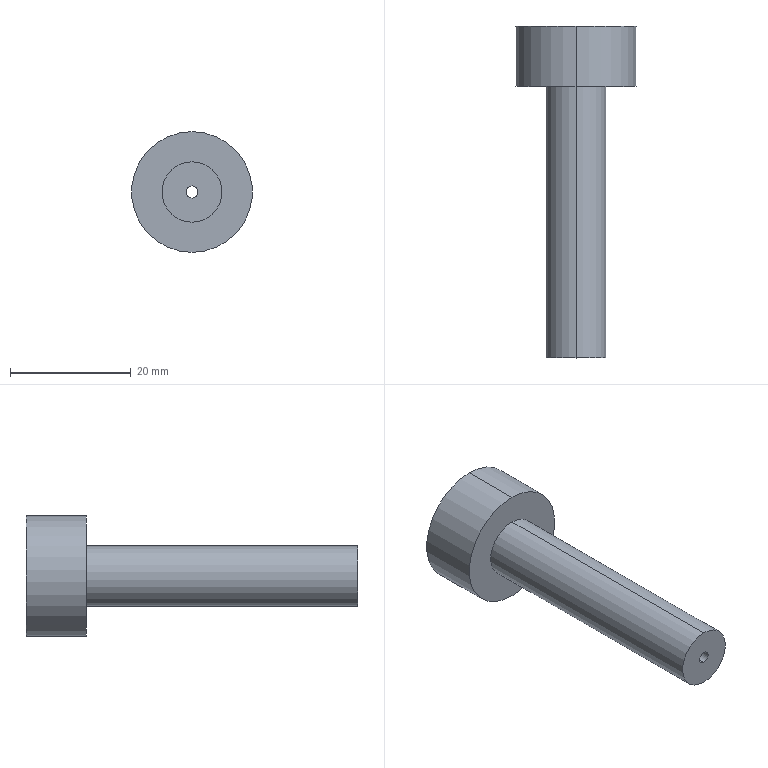Part | 1 solid | 16 faces | box 20 x 55 x 20 mm | volume 5586 mm3 | cylinder 10 | plane 4 | cone 2 | commonest cylinder face diameters 2 x4 6 x2 10 x2 20 x2
STEP:
#1=CARTESIAN_POINT('',(0.,-2.8,-1.));
#2=VERTEX_POINT('',#1);
#3=CARTESIAN_POINT('',(-1.,-2.8,0.));
#4=VERTEX_POINT('',#3);
#5=CARTESIAN_POINT('',(0.,-2.8,0.));
#6=DIRECTION('',(0.,1.,0.));
#7=DIRECTION('',(-1.,0.,0.));
#8=AXIS2_PLACEMENT_3D('',#5,#6,#7);
#9=CIRCLE('',#8,1.);
#10=EDGE_CURVE('',#2,#4,#9,.T.);
#11=ORIENTED_EDGE('',*,*,#10,.T.);
#12=CARTESIAN_POINT('',(-3.,-4.,0.));
#13=VERTEX_POINT('',#12);
#14=CARTESIAN_POINT('',(-1.,-2.8,0.));
#15=DIRECTION('',(-0.8575,-0.5145,0.));
#16=VECTOR('',#15,1000.);
#17=LINE('',#14,#16);
#18=EDGE_CURVE('',#4,#13,#17,.T.);
#19=ORIENTED_EDGE('',*,*,#18,.T.);
#20=CARTESIAN_POINT('',(0.,-4.,-3.));
#21=VERTEX_POINT('',#20);
#22=CARTESIAN_POINT('',(0.,-4.,0.));
#23=DIRECTION('',(0.,1.,0.));
#24=DIRECTION('',(-1.,0.,0.));
#25=AXIS2_PLACEMENT_3D('',#22,#23,#24);
#26=CIRCLE('',#25,3.);
#27=EDGE_CURVE('',#21,#13,#26,.T.);
#28=ORIENTED_EDGE('',*,*,#27,.F.);
#29=CARTESIAN_POINT('',(3.,-4.,0.));
#30=VERTEX_POINT('',#29);
#31=CARTESIAN_POINT('',(0.,-4.,0.));
#32=DIRECTION('',(0.,1.,0.));
#33=DIRECTION('',(-1.,0.,0.));
#34=AXIS2_PLACEMENT_3D('',#31,#32,#33);
#35=CIRCLE('',#34,3.);
#36=EDGE_CURVE('',#30,#21,#35,.T.);
#37=ORIENTED_EDGE('',*,*,#36,.F.);
#38=CARTESIAN_POINT('',(1.,-2.8,0.));
#39=VERTEX_POINT('',#38);
#40=CARTESIAN_POINT('',(1.,-2.8,0.));
#41=DIRECTION('',(0.8575,-0.5145,0.));
#42=VECTOR('',#41,1000.);
#43=LINE('',#40,#42);
#44=EDGE_CURVE('',#39,#30,#43,.T.);
#45=ORIENTED_EDGE('',*,*,#44,.F.);
#46=CARTESIAN_POINT('',(0.,-2.8,0.));
#47=DIRECTION('',(0.,1.,0.));
#48=DIRECTION('',(-1.,0.,0.));
#49=AXIS2_PLACEMENT_3D('',#46,#47,#48);
#50=CIRCLE('',#49,1.);
#51=EDGE_CURVE('',#39,#2,#50,.T.);
#52=ORIENTED_EDGE('',*,*,#51,.T.);
#53=EDGE_LOOP('',(#11,#19,#28,#37,#45,#52));
#54=FACE_OUTER_BOUND('',#53,.T.);
#55=CARTESIAN_POINT('',(0.,-2.8,0.));
#56=DIRECTION('',(0.,-1.,0.));
#57=DIRECTION('',(1.,0.,0.));
#58=AXIS2_PLACEMENT_3D('',#55,#56,#57);
#59=CONICAL_SURFACE('',#58,1.,1.03);
#60=ADVANCED_FACE('',(#54),#59,.F.);
#61=ORIENTED_EDGE('',*,*,#27,.T.);
#62=CARTESIAN_POINT('',(0.,-4.,3.));
#63=VERTEX_POINT('',#62);
#64=CARTESIAN_POINT('',(0.,-4.,0.));
#65=DIRECTION('',(0.,1.,0.));
#66=DIRECTION('',(-1.,0.,0.));
#67=AXIS2_PLACEMENT_3D('',#64,#65,#66);
#68=CIRCLE('',#67,3.);
#69=EDGE_CURVE('',#13,#63,#68,.T.);
#70=ORIENTED_EDGE('',*,*,#69,.T.);
#71=CARTESIAN_POINT('',(0.,-40.,3.));
#72=VERTEX_POINT('',#71);
#73=CARTESIAN_POINT('',(0.,-4.,3.));
#74=DIRECTION('',(0.,-1.,0.));
#75=VECTOR('',#74,1000.);
#76=LINE('',#73,#75);
#77=EDGE_CURVE('',#63,#72,#76,.T.);
#78=ORIENTED_EDGE('',*,*,#77,.T.);
#79=CARTESIAN_POINT('',(0.,-40.,-3.));
#80=VERTEX_POINT('',#79);
#81=CARTESIAN_POINT('',(0.,-40.,0.));
#82=DIRECTION('',(0.,-1.,0.));
#83=DIRECTION('',(0.,0.,-1.));
#84=AXIS2_PLACEMENT_3D('',#81,#82,#83);
#85=CIRCLE('',#84,3.);
#86=EDGE_CURVE('',#72,#80,#85,.T.);
#87=ORIENTED_EDGE('',*,*,#86,.T.);
#88=CARTESIAN_POINT('',(0.,-4.,-3.));
#89=DIRECTION('',(0.,-1.,0.));
#90=VECTOR('',#89,1000.);
#91=LINE('',#88,#90);
#92=EDGE_CURVE('',#21,#80,#91,.T.);
#93=ORIENTED_EDGE('',*,*,#92,.F.);
#94=EDGE_LOOP('',(#61,#70,#78,#87,#93));
#95=FACE_OUTER_BOUND('',#94,.T.);
#96=CARTESIAN_POINT('',(0.,-4.,0.));
#97=DIRECTION('',(0.,-1.,0.));
#98=DIRECTION('',(0.,0.,-1.));
#99=AXIS2_PLACEMENT_3D('',#96,#97,#98);
#100=CYLINDRICAL_SURFACE('',#99,3.);
#101=ADVANCED_FACE('',(#95),#100,.F.);
#102=CARTESIAN_POINT('',(0.,-45.,-1.));
#103=VERTEX_POINT('',#102);
#104=CARTESIAN_POINT('',(0.,-45.,1.));
#105=VERTEX_POINT('',#104);
#106=CARTESIAN_POINT('',(0.,-45.,0.));
#107=DIRECTION('',(0.,1.,0.));
#108=DIRECTION('',(0.,0.,1.));
#109=AXIS2_PLACEMENT_3D('',#106,#107,#108);
#110=CIRCLE('',#109,1.);
#111=EDGE_CURVE('',#103,#105,#110,.T.);
#112=ORIENTED_EDGE('',*,*,#111,.F.);
#113=CARTESIAN_POINT('',(0.,-40.,-1.));
#114=VERTEX_POINT('',#113);
#115=CARTESIAN_POINT('',(0.,-45.,-1.));
#116=DIRECTION('',(0.,1.,0.));
#117=VECTOR('',#116,1000.);
#118=LINE('',#115,#117);
#119=EDGE_CURVE('',#103,#114,#118,.T.);
#120=ORIENTED_EDGE('',*,*,#119,.T.);
#121=CARTESIAN_POINT('',(0.,-40.,1.));
#122=VERTEX_POINT('',#121);
#123=CARTESIAN_POINT('',(0.,-40.,0.));
#124=DIRECTION('',(0.,1.,0.));
#125=DIRECTION('',(0.,0.,-1.));
#126=AXIS2_PLACEMENT_3D('',#123,#124,#125);
#127=CIRCLE('',#126,1.);
#128=EDGE_CURVE('',#114,#122,#127,.T.);
#129=ORIENTED_EDGE('',*,*,#128,.T.);
#130=CARTESIAN_POINT('',(0.,-45.,1.));
#131=DIRECTION('',(0.,1.,0.));
#132=VECTOR('',#131,1000.);
#133=LINE('',#130,#132);
#134=EDGE_CURVE('',#105,#122,#133,.T.);
#135=ORIENTED_EDGE('',*,*,#134,.F.);
#136=EDGE_LOOP('',(#112,#120,#129,#135));
#137=FACE_OUTER_BOUND('',#136,.T.);
#138=CARTESIAN_POINT('',(0.,-45.,0.));
#139=DIRECTION('',(0.,1.,0.));
#140=DIRECTION('',(0.,0.,1.));
#141=AXIS2_PLACEMENT_3D('',#138,#139,#140);
#142=CYLINDRICAL_SURFACE('',#141,1.);
#143=ADVANCED_FACE('',(#137),#142,.F.);
#144=CARTESIAN_POINT('',(0.,-45.,-5.));
#145=VERTEX_POINT('',#144);
#146=CARTESIAN_POINT('',(0.,-45.,5.));
#147=VERTEX_POINT('',#146);
#148=CARTESIAN_POINT('',(0.,-45.,0.));
#149=DIRECTION('',(0.,-1.,0.));
#150=DIRECTION('',(0.,0.,-1.));
#151=AXIS2_PLACEMENT_3D('',#148,#149,#150);
#152=CIRCLE('',#151,5.);
#153=EDGE_CURVE('',#145,#147,#152,.T.);
#154=ORIENTED_EDGE('',*,*,#153,.F.);
#155=CARTESIAN_POINT('',(0.,0.,-5.));
#156=VERTEX_POINT('',#155);
#157=CARTESIAN_POINT('',(0.,-45.,-5.));
#158=DIRECTION('',(0.,1.,0.));
#159=VECTOR('',#158,1000.);
#160=LINE('',#157,#159);
#161=EDGE_CURVE('',#145,#156,#160,.T.);
#162=ORIENTED_EDGE('',*,*,#161,.T.);
#163=CARTESIAN_POINT('',(0.,0.,5.));
#164=VERTEX_POINT('',#163);
#165=CARTESIAN_POINT('',(0.,0.,0.));
#166=DIRECTION('',(0.,-1.,0.));
#167=DIRECTION('',(0.,0.,-1.));
#168=AXIS2_PLACEMENT_3D('',#165,#166,#167);
#169=CIRCLE('',#168,5.);
#170=EDGE_CURVE('',#156,#164,#169,.T.);
#171=ORIENTED_EDGE('',*,*,#170,.T.);
#172=CARTESIAN_POINT('',(0.,-45.,5.));
#173=DIRECTION('',(0.,1.,0.));
#174=VECTOR('',#173,1000.);
#175=LINE('',#172,#174);
#176=EDGE_CURVE('',#147,#164,#175,.T.);
#177=ORIENTED_EDGE('',*,*,#176,.F.);
#178=EDGE_LOOP('',(#154,#162,#171,#177));
#179=FACE_OUTER_BOUND('',#178,.T.);
#180=CARTESIAN_POINT('',(0.,-45.,0.));
#181=DIRECTION('',(0.,1.,0.));
#182=DIRECTION('',(0.,0.,1.));
#183=AXIS2_PLACEMENT_3D('',#180,#181,#182);
#184=CYLINDRICAL_SURFACE('',#183,5.);
#185=ADVANCED_FACE('',(#179),#184,.T.);
#186=CARTESIAN_POINT('',(0.,10.,10.));
#187=VERTEX_POINT('',#186);
#188=CARTESIAN_POINT('',(0.,10.,-10.));
#189=VERTEX_POINT('',#188);
#190=CARTESIAN_POINT('',(0.,10.,0.));
#191=DIRECTION('',(0.,1.,0.));
#192=DIRECTION('',(0.,0.,1.));
#193=AXIS2_PLACEMENT_3D('',#190,#191,#192);
#194=CIRCLE('',#193,10.);
#195=EDGE_CURVE('',#187,#189,#194,.T.);
#196=ORIENTED_EDGE('',*,*,#195,.F.);
#197=CARTESIAN_POINT('',(0.,0.,10.));
#198=VERTEX_POINT('',#197);
#199=CARTESIAN_POINT('',(0.,10.,10.));
#200=DIRECTION('',(0.,-1.,0.));
#201=VECTOR('',#200,1000.);
#202=LINE('',#199,#201);
#203=EDGE_CURVE('',#187,#198,#202,.T.);
#204=ORIENTED_EDGE('',*,*,#203,.T.);
#205=CARTESIAN_POINT('',(0.,0.,-10.));
#206=VERTEX_POINT('',#205);
#207=CARTESIAN_POINT('',(0.,0.,0.));
#208=DIRECTION('',(0.,1.,0.));
#209=DIRECTION('',(0.,0.,1.));
#210=AXIS2_PLACEMENT_3D('',#207,#208,#209);
#211=CIRCLE('',#210,10.);
#212=EDGE_CURVE('',#198,#206,#211,.T.);
#213=ORIENTED_EDGE('',*,*,#212,.T.);
#214=CARTESIAN_POINT('',(0.,10.,-10.));
#215=DIRECTION('',(0.,-1.,0.));
#216=VECTOR('',#215,1000.);
#217=LINE('',#214,#216);
#218=EDGE_CURVE('',#189,#206,#217,.T.);
#219=ORIENTED_EDGE('',*,*,#218,.F.);
#220=EDGE_LOOP('',(#196,#204,#213,#219));
#221=FACE_OUTER_BOUND('',#220,.T.);
#222=CARTESIAN_POINT('',(0.,10.,0.));
#223=DIRECTION('',(0.,-1.,0.));
#224=DIRECTION('',(0.,0.,-1.));
#225=AXIS2_PLACEMENT_3D('',#222,#223,#224);
#226=CYLINDRICAL_SURFACE('',#225,10.);
#227=ADVANCED_FACE('',(#221),#226,.T.);
#228=ORIENTED_EDGE('',*,*,#10,.F.);
#229=CARTESIAN_POINT('',(0.,10.,-1.));
#230=VERTEX_POINT('',#229);
#231=CARTESIAN_POINT('',(0.,-45.,-1.));
#232=DIRECTION('',(0.,1.,0.));
#233=VECTOR('',#232,1000.);
#234=LINE('',#231,#233);
#235=EDGE_CURVE('',#2,#230,#234,.T.);
#236=ORIENTED_EDGE('',*,*,#235,.T.);
#237=CARTESIAN_POINT('',(0.,10.,1.));
#238=VERTEX_POINT('',#237);
#239=CARTESIAN_POINT('',(0.,10.,0.));
#240=DIRECTION('',(0.,1.,0.));
#241=DIRECTION('',(0.,0.,1.));
#242=AXIS2_PLACEMENT_3D('',#239,#240,#241);
#243=CIRCLE('',#242,1.);
#244=EDGE_CURVE('',#230,#238,#243,.T.);
#245=ORIENTED_EDGE('',*,*,#244,.T.);
#246=CARTESIAN_POINT('',(0.,-2.8,1.));
#247=VERTEX_POINT('',#246);
#248=CARTESIAN_POINT('',(0.,-45.,1.));
#249=DIRECTION('',(0.,1.,0.));
#250=VECTOR('',#249,1000.);
#251=LINE('',#248,#250);
#252=EDGE_CURVE('',#247,#238,#251,.T.);
#253=ORIENTED_EDGE('',*,*,#252,.F.);
#254=CARTESIAN_POINT('',(0.,-2.8,0.));
#255=DIRECTION('',(0.,1.,0.));
#256=DIRECTION('',(-1.,0.,0.));
#257=AXIS2_PLACEMENT_3D('',#254,#255,#256);
#258=CIRCLE('',#257,1.);
#259=EDGE_CURVE('',#4,#247,#258,.T.);
#260=ORIENTED_EDGE('',*,*,#259,.F.);
#261=EDGE_LOOP('',(#228,#236,#245,#253,#260));
#262=FACE_OUTER_BOUND('',#261,.T.);
#263=CARTESIAN_POINT('',(0.,-45.,0.));
#264=DIRECTION('',(0.,1.,0.));
#265=DIRECTION('',(0.,0.,1.));
#266=AXIS2_PLACEMENT_3D('',#263,#264,#265);
#267=CYLINDRICAL_SURFACE('',#266,1.);
#268=ADVANCED_FACE('',(#262),#267,.F.);
#269=ORIENTED_EDGE('',*,*,#235,.F.);
#270=ORIENTED_EDGE('',*,*,#51,.F.);
#271=CARTESIAN_POINT('',(0.,-2.8,0.));
#272=DIRECTION('',(0.,1.,0.));
#273=DIRECTION('',(-1.,0.,0.));
#274=AXIS2_PLACEMENT_3D('',#271,#272,#273);
#275=CIRCLE('',#274,1.);
#276=EDGE_CURVE('',#247,#39,#275,.T.);
#277=ORIENTED_EDGE('',*,*,#276,.F.);
#278=ORIENTED_EDGE('',*,*,#252,.T.);
#279=CARTESIAN_POINT('',(0.,10.,0.));
#280=DIRECTION('',(0.,1.,0.));
#281=DIRECTION('',(0.,0.,1.));
#282=AXIS2_PLACEMENT_3D('',#279,#280,#281);
#283=CIRCLE('',#282,1.);
#284=EDGE_CURVE('',#238,#230,#283,.T.);
#285=ORIENTED_EDGE('',*,*,#284,.T.);
#286=EDGE_LOOP('',(#269,#270,#277,#278,#285));
#287=FACE_OUTER_BOUND('',#286,.T.);
#288=CARTESIAN_POINT('',(0.,-45.,0.));
#289=DIRECTION('',(0.,1.,0.));
#290=DIRECTION('',(0.,0.,1.));
#291=AXIS2_PLACEMENT_3D('',#288,#289,#290);
#292=CYLINDRICAL_SURFACE('',#291,1.);
#293=ADVANCED_FACE('',(#287),#292,.F.);
#294=ORIENTED_EDGE('',*,*,#203,.F.);
#295=CARTESIAN_POINT('',(0.,10.,0.));
#296=DIRECTION('',(0.,1.,0.));
#297=DIRECTION('',(0.,0.,1.));
#298=AXIS2_PLACEMENT_3D('',#295,#296,#297);
#299=CIRCLE('',#298,10.);
#300=EDGE_CURVE('',#189,#187,#299,.T.);
#301=ORIENTED_EDGE('',*,*,#300,.F.);
#302=ORIENTED_EDGE('',*,*,#218,.T.);
#303=CARTESIAN_POINT('',(0.,0.,0.));
#304=DIRECTION('',(0.,1.,0.));
#305=DIRECTION('',(0.,0.,1.));
#306=AXIS2_PLACEMENT_3D('',#303,#304,#305);
#307=CIRCLE('',#306,10.);
#308=EDGE_CURVE('',#206,#198,#307,.T.);
#309=ORIENTED_EDGE('',*,*,#308,.T.);
#310=EDGE_LOOP('',(#294,#301,#302,#309));
#311=FACE_OUTER_BOUND('',#310,.T.);
#312=CARTESIAN_POINT('',(0.,10.,0.));
#313=DIRECTION('',(0.,-1.,0.));
#314=DIRECTION('',(0.,0.,-1.));
#315=AXIS2_PLACEMENT_3D('',#312,#313,#314);
#316=CYLINDRICAL_SURFACE('',#315,10.);
#317=ADVANCED_FACE('',(#311),#316,.T.);
#318=ORIENTED_EDGE('',*,*,#284,.F.);
#319=ORIENTED_EDGE('',*,*,#244,.F.);
#320=EDGE_LOOP('',(#318,#319));
#321=FACE_BOUND('',#320,.T.);
#322=ORIENTED_EDGE('',*,*,#300,.T.);
#323=ORIENTED_EDGE('',*,*,#195,.T.);
#324=EDGE_LOOP('',(#322,#323));
#325=FACE_OUTER_BOUND('',#324,.T.);
#326=CARTESIAN_POINT('',(0.,10.,0.));
#327=DIRECTION('',(0.,1.,0.));
#328=DIRECTION('',(0.,0.,1.));
#329=AXIS2_PLACEMENT_3D('',#326,#327,#328);
#330=PLANE('',#329);
#331=ADVANCED_FACE('',(#321,#325),#330,.T.);
#332=CARTESIAN_POINT('',(0.,0.,0.));
#333=DIRECTION('',(0.,-1.,0.));
#334=DIRECTION('',(0.,0.,-1.));
#335=AXIS2_PLACEMENT_3D('',#332,#333,#334);
#336=CIRCLE('',#335,5.);
#337=EDGE_CURVE('',#164,#156,#336,.T.);
#338=ORIENTED_EDGE('',*,*,#337,.F.);
#339=ORIENTED_EDGE('',*,*,#170,.F.);
#340=EDGE_LOOP('',(#338,#339));
#341=FACE_BOUND('',#340,.T.);
#342=ORIENTED_EDGE('',*,*,#308,.F.);
#343=ORIENTED_EDGE('',*,*,#212,.F.);
#344=EDGE_LOOP('',(#342,#343));
#345=FACE_OUTER_BOUND('',#344,.T.);
#346=CARTESIAN_POINT('',(0.,0.,0.));
#347=DIRECTION('',(0.,1.,0.));
#348=DIRECTION('',(0.,0.,1.));
#349=AXIS2_PLACEMENT_3D('',#346,#347,#348);
#350=PLANE('',#349);
#351=ADVANCED_FACE('',(#341,#345),#350,.F.);
#352=ORIENTED_EDGE('',*,*,#161,.F.);
#353=CARTESIAN_POINT('',(0.,-45.,0.));
#354=DIRECTION('',(0.,-1.,0.));
#355=DIRECTION('',(0.,0.,-1.));
#356=AXIS2_PLACEMENT_3D('',#353,#354,#355);
#357=CIRCLE('',#356,5.);
#358=EDGE_CURVE('',#147,#145,#357,.T.);
#359=ORIENTED_EDGE('',*,*,#358,.F.);
#360=ORIENTED_EDGE('',*,*,#176,.T.);
#361=ORIENTED_EDGE('',*,*,#337,.T.);
#362=EDGE_LOOP('',(#352,#359,#360,#361));
#363=FACE_OUTER_BOUND('',#362,.T.);
#364=CARTESIAN_POINT('',(0.,-45.,0.));
#365=DIRECTION('',(0.,1.,0.));
#366=DIRECTION('',(0.,0.,1.));
#367=AXIS2_PLACEMENT_3D('',#364,#365,#366);
#368=CYLINDRICAL_SURFACE('',#367,5.);
#369=ADVANCED_FACE('',(#363),#368,.T.);
#370=CARTESIAN_POINT('',(0.,-45.,0.));
#371=DIRECTION('',(0.,1.,0.));
#372=DIRECTION('',(0.,0.,1.));
#373=AXIS2_PLACEMENT_3D('',#370,#371,#372);
#374=CIRCLE('',#373,1.);
#375=EDGE_CURVE('',#105,#103,#374,.T.);
#376=ORIENTED_EDGE('',*,*,#375,.T.);
#377=ORIENTED_EDGE('',*,*,#111,.T.);
#378=EDGE_LOOP('',(#376,#377));
#379=FACE_BOUND('',#378,.T.);
#380=ORIENTED_EDGE('',*,*,#358,.T.);
#381=ORIENTED_EDGE('',*,*,#153,.T.);
#382=EDGE_LOOP('',(#380,#381));
#383=FACE_OUTER_BOUND('',#382,.T.);
#384=CARTESIAN_POINT('',(0.,-45.,0.));
#385=DIRECTION('',(0.,-1.,0.));
#386=DIRECTION('',(0.,0.,-1.));
#387=AXIS2_PLACEMENT_3D('',#384,#385,#386);
#388=PLANE('',#387);
#389=ADVANCED_FACE('',(#379,#383),#388,.T.);
#390=ORIENTED_EDGE('',*,*,#119,.F.);
#391=ORIENTED_EDGE('',*,*,#375,.F.);
#392=ORIENTED_EDGE('',*,*,#134,.T.);
#393=CARTESIAN_POINT('',(0.,-40.,0.));
#394=DIRECTION('',(0.,1.,0.));
#395=DIRECTION('',(0.,0.,-1.));
#396=AXIS2_PLACEMENT_3D('',#393,#394,#395);
#397=CIRCLE('',#396,1.);
#398=EDGE_CURVE('',#122,#114,#397,.T.);
#399=ORIENTED_EDGE('',*,*,#398,.T.);
#400=EDGE_LOOP('',(#390,#391,#392,#399));
#401=FACE_OUTER_BOUND('',#400,.T.);
#402=CARTESIAN_POINT('',(0.,-45.,0.));
#403=DIRECTION('',(0.,1.,0.));
#404=DIRECTION('',(0.,0.,1.));
#405=AXIS2_PLACEMENT_3D('',#402,#403,#404);
#406=CYLINDRICAL_SURFACE('',#405,1.);
#407=ADVANCED_FACE('',(#401),#406,.F.);
#408=CARTESIAN_POINT('',(0.,-40.,0.));
#409=DIRECTION('',(0.,-1.,0.));
#410=DIRECTION('',(0.,0.,-1.));
#411=AXIS2_PLACEMENT_3D('',#408,#409,#410);
#412=CIRCLE('',#411,3.);
#413=EDGE_CURVE('',#80,#72,#412,.T.);
#414=ORIENTED_EDGE('',*,*,#413,.F.);
#415=ORIENTED_EDGE('',*,*,#86,.F.);
#416=EDGE_LOOP('',(#414,#415));
#417=FACE_OUTER_BOUND('',#416,.T.);
#418=ORIENTED_EDGE('',*,*,#398,.F.);
#419=ORIENTED_EDGE('',*,*,#128,.F.);
#420=EDGE_LOOP('',(#418,#419));
#421=FACE_BOUND('',#420,.T.);
#422=CARTESIAN_POINT('',(0.,-40.,0.));
#423=DIRECTION('',(0.,-1.,0.));
#424=DIRECTION('',(0.,0.,-1.));
#425=AXIS2_PLACEMENT_3D('',#422,#423,#424);
#426=PLANE('',#425);
#427=ADVANCED_FACE('',(#417,#421),#426,.F.);
#428=ORIENTED_EDGE('',*,*,#77,.F.);
#429=CARTESIAN_POINT('',(0.,-4.,0.));
#430=DIRECTION('',(0.,1.,0.));
#431=DIRECTION('',(-1.,0.,0.));
#432=AXIS2_PLACEMENT_3D('',#429,#430,#431);
#433=CIRCLE('',#432,3.);
#434=EDGE_CURVE('',#63,#30,#433,.T.);
#435=ORIENTED_EDGE('',*,*,#434,.T.);
#436=ORIENTED_EDGE('',*,*,#36,.T.);
#437=ORIENTED_EDGE('',*,*,#92,.T.);
#438=ORIENTED_EDGE('',*,*,#413,.T.);
#439=EDGE_LOOP('',(#428,#435,#436,#437,#438));
#440=FACE_OUTER_BOUND('',#439,.T.);
#441=CARTESIAN_POINT('',(0.,-4.,0.));
#442=DIRECTION('',(0.,-1.,0.));
#443=DIRECTION('',(0.,0.,-1.));
#444=AXIS2_PLACEMENT_3D('',#441,#442,#443);
#445=CYLINDRICAL_SURFACE('',#444,3.);
#446=ADVANCED_FACE('',(#440),#445,.F.);
#447=ORIENTED_EDGE('',*,*,#18,.F.);
#448=ORIENTED_EDGE('',*,*,#259,.T.);
#449=ORIENTED_EDGE('',*,*,#276,.T.);
#450=ORIENTED_EDGE('',*,*,#44,.T.);
#451=ORIENTED_EDGE('',*,*,#434,.F.);
#452=ORIENTED_EDGE('',*,*,#69,.F.);
#453=EDGE_LOOP('',(#447,#448,#449,#450,#451,#452));
#454=FACE_OUTER_BOUND('',#453,.T.);
#455=CARTESIAN_POINT('',(0.,-2.8,0.));
#456=DIRECTION('',(0.,-1.,0.));
#457=DIRECTION('',(1.,0.,0.));
#458=AXIS2_PLACEMENT_3D('',#455,#456,#457);
#459=CONICAL_SURFACE('',#458,1.,1.03);
#460=ADVANCED_FACE('',(#454),#459,.F.);
#461=CLOSED_SHELL('',(#60,#101,#143,#185,#227,#268,#293,#317,#331,#351,#369,#389,#407,#427,#446,#460));
#462=MANIFOLD_SOLID_BREP('',#461);
#463=CARTESIAN_POINT('',(0.,0.,0.));
#464=DIRECTION('',(0.,0.,1.));
#465=DIRECTION('',(1.,0.,0.));
#466=AXIS2_PLACEMENT_3D('',#463,#464,#465);
#467=(LENGTH_UNIT()NAMED_UNIT(*)SI_UNIT(.MILLI.,.METRE.));
#468=UNCERTAINTY_MEASURE_WITH_UNIT(LENGTH_MEASURE(0.00001),#467,'','');
#469=(NAMED_UNIT(*)PLANE_ANGLE_UNIT()SI_UNIT($,.RADIAN.));
#470=(NAMED_UNIT(*)SI_UNIT($,.STERADIAN.)SOLID_ANGLE_UNIT());
#471=(GEOMETRIC_REPRESENTATION_CONTEXT(3)GLOBAL_UNCERTAINTY_ASSIGNED_CONTEXT((#468))GLOBAL_UNIT_ASSIGNED_CONTEXT((#467,#469,#470))REPRESENTATION_CONTEXT('',''));
#472=ADVANCED_BREP_SHAPE_REPRESENTATION('',(#462,#466),#471);